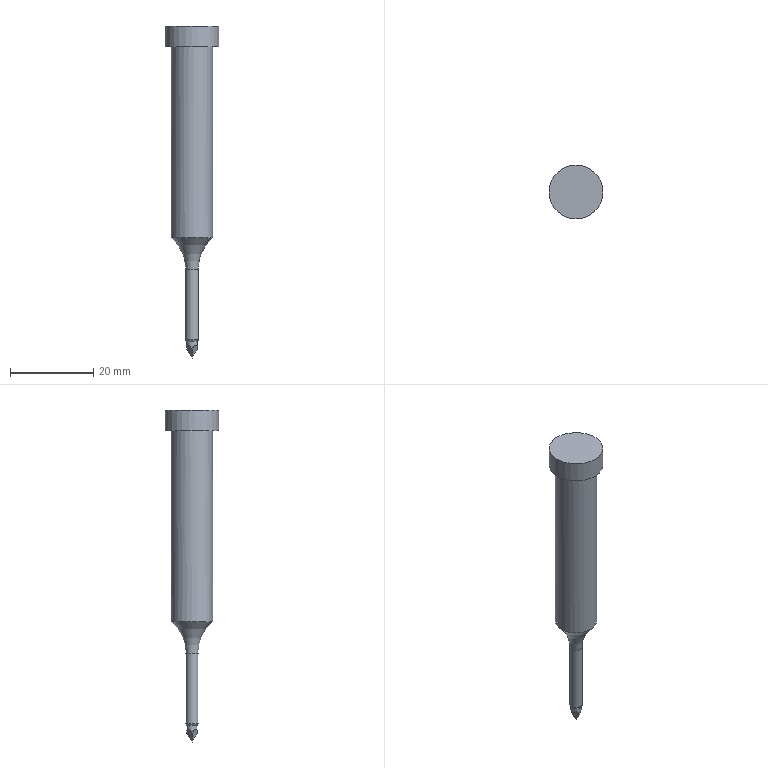Part | NX | features solid 2 | 1 solid | 13 faces | box 13 x 13 x 80 mm | volume 4592 mm3 | plane 7 | cylinder 4 | torus 2 | commonest cylinder face diameters 2.5 x1 3.006 x1 10 x1 13 x1
STEP:
#1=CARTESIAN_POINT('',(516.232,-362.056,-63.597));
#2=VERTEX_POINT('',#1);
#3=CARTESIAN_POINT('',(517.735,-362.056,-63.597));
#4=DIRECTION('',(0.,0.,-1.));
#5=DIRECTION('',(-1.,0.,0.));
#6=AXIS2_PLACEMENT_3D('',#3,#4,#5);
#7=CIRCLE('',#6,1.503);
#8=EDGE_CURVE('',#2,#2,#7,.F.);
#9=ORIENTED_EDGE('',*,*,#8,.F.);
#10=EDGE_LOOP('',(#9));
#11=FACE_BOUND('',#10,.T.);
#12=CARTESIAN_POINT('',(519.238,-362.056,-80.5));
#13=VERTEX_POINT('',#12);
#14=CARTESIAN_POINT('',(517.735,-362.056,-80.5));
#15=DIRECTION('',(0.,0.,1.));
#16=DIRECTION('',(1.,0.,0.));
#17=AXIS2_PLACEMENT_3D('',#14,#15,#16);
#18=CIRCLE('',#17,1.503);
#19=EDGE_CURVE('',#13,#13,#18,.F.);
#20=ORIENTED_EDGE('',*,*,#19,.F.);
#21=EDGE_LOOP('',(#20));
#22=FACE_BOUND('',#21,.T.);
#23=CARTESIAN_POINT('',(517.735,-362.056,-60.));
#24=DIRECTION('',(0.,0.,-1.));
#25=DIRECTION('',(1.,0.,0.));
#26=AXIS2_PLACEMENT_3D('',#23,#24,#25);
#27=CYLINDRICAL_SURFACE('',#26,1.503);
#28=ADVANCED_FACE('',(#11,#22),#27,.T.);
#29=ORIENTED_EDGE('',*,*,#19,.T.);
#30=EDGE_LOOP('',(#29));
#31=FACE_BOUND('',#30,.T.);
#32=CARTESIAN_POINT('',(518.738,-362.056,-81.));
#33=VERTEX_POINT('',#32);
#34=CARTESIAN_POINT('',(517.735,-362.056,-81.));
#35=DIRECTION('',(0.,0.,1.));
#36=DIRECTION('',(1.,0.,0.));
#37=AXIS2_PLACEMENT_3D('',#34,#35,#36);
#38=CIRCLE('',#37,1.003);
#39=EDGE_CURVE('',#33,#33,#38,.T.);
#40=ORIENTED_EDGE('',*,*,#39,.T.);
#41=EDGE_LOOP('',(#40));
#42=FACE_BOUND('',#41,.T.);
#43=CARTESIAN_POINT('',(517.735,-362.056,-80.5));
#44=DIRECTION('',(0.,0.,-1.));
#45=DIRECTION('',(1.,0.,0.));
#46=AXIS2_PLACEMENT_3D('',#43,#44,#45);
#47=TOROIDAL_SURFACE('',#46,1.003,0.5);
#48=ADVANCED_FACE('',(#31,#42),#47,.T.);
#49=CARTESIAN_POINT('',(522.735,-362.056,-56.));
#50=VERTEX_POINT('',#49);
#51=CARTESIAN_POINT('',(517.735,-362.056,-56.));
#52=DIRECTION('',(0.,0.,1.));
#53=DIRECTION('',(1.,0.,0.));
#54=AXIS2_PLACEMENT_3D('',#51,#52,#53);
#55=CIRCLE('',#54,5.);
#56=EDGE_CURVE('',#50,#50,#55,.T.);
#57=ORIENTED_EDGE('',*,*,#56,.F.);
#58=EDGE_LOOP('',(#57));
#59=FACE_BOUND('',#58,.T.);
#60=ORIENTED_EDGE('',*,*,#8,.T.);
#61=EDGE_LOOP('',(#60));
#62=FACE_BOUND('',#61,.T.);
#63=CARTESIAN_POINT('',(517.735,-362.056,-63.597));
#64=DIRECTION('',(0.,0.,1.));
#65=DIRECTION('',(-1.,0.,0.));
#66=AXIS2_PLACEMENT_3D('',#63,#64,#65);
#67=TOROIDAL_SURFACE('',#66,11.503,10.);
#68=ADVANCED_FACE('',(#59,#62),#67,.F.);
#69=CARTESIAN_POINT('',(518.985,-362.056,-81.));
#70=VERTEX_POINT('',#69);
#71=CARTESIAN_POINT('',(517.735,-362.056,-81.));
#72=DIRECTION('',(0.,0.,1.));
#73=DIRECTION('',(1.,0.,0.));
#74=AXIS2_PLACEMENT_3D('',#71,#72,#73);
#75=CIRCLE('',#74,1.25);
#76=EDGE_CURVE('',#70,#70,#75,.T.);
#77=ORIENTED_EDGE('',*,*,#76,.F.);
#78=EDGE_LOOP('',(#77));
#79=FACE_BOUND('',#78,.T.);
#80=CARTESIAN_POINT('',(518.985,-362.056,-82.835));
#81=VERTEX_POINT('',#80);
#82=CARTESIAN_POINT('',(517.735,-363.306,-82.835));
#83=VERTEX_POINT('',#82);
#84=CARTESIAN_POINT('',(517.735,-362.056,-85.));
#85=DIRECTION('',(0.6547,-0.6547,-0.378));
#86=DIRECTION('',(0.2673,-0.2673,0.9258));
#87=AXIS2_PLACEMENT_3D('',#84,#85,#86);
#88=ELLIPSE('',#87,3.307,1.25);
#89=EDGE_CURVE('',#81,#83,#88,.T.);
#90=ORIENTED_EDGE('',*,*,#89,.F.);
#91=CARTESIAN_POINT('',(517.735,-360.806,-82.835));
#92=VERTEX_POINT('',#91);
#93=CARTESIAN_POINT('',(517.735,-362.056,-85.));
#94=DIRECTION('',(0.6547,0.6547,-0.378));
#95=DIRECTION('',(0.2673,0.2673,0.9258));
#96=AXIS2_PLACEMENT_3D('',#93,#94,#95);
#97=ELLIPSE('',#96,3.307,1.25);
#98=EDGE_CURVE('',#92,#81,#97,.T.);
#99=ORIENTED_EDGE('',*,*,#98,.F.);
#100=CARTESIAN_POINT('',(516.485,-362.056,-82.835));
#101=VERTEX_POINT('',#100);
#102=CARTESIAN_POINT('',(517.735,-362.056,-85.));
#103=DIRECTION('',(0.6547,-0.6547,0.378));
#104=DIRECTION('',(-0.2673,0.2673,0.9258));
#105=AXIS2_PLACEMENT_3D('',#102,#103,#104);
#106=ELLIPSE('',#105,3.307,1.25);
#107=EDGE_CURVE('',#92,#101,#106,.T.);
#108=ORIENTED_EDGE('',*,*,#107,.T.);
#109=CARTESIAN_POINT('',(517.735,-362.056,-85.));
#110=DIRECTION('',(-0.6547,-0.6547,-0.378));
#111=DIRECTION('',(-0.2673,-0.2673,0.9258));
#112=AXIS2_PLACEMENT_3D('',#109,#110,#111);
#113=ELLIPSE('',#112,3.307,1.25);
#114=EDGE_CURVE('',#83,#101,#113,.T.);
#115=ORIENTED_EDGE('',*,*,#114,.F.);
#116=EDGE_LOOP('',(#90,#99,#108,#115));
#117=FACE_BOUND('',#116,.T.);
#118=CARTESIAN_POINT('',(517.735,-362.056,-85.));
#119=DIRECTION('',(0.,0.,1.));
#120=DIRECTION('',(-1.,0.,0.));
#121=AXIS2_PLACEMENT_3D('',#118,#119,#120);
#122=CYLINDRICAL_SURFACE('',#121,1.25);
#123=ADVANCED_FACE('',(#79,#117),#122,.T.);
#124=ORIENTED_EDGE('',*,*,#39,.F.);
#125=EDGE_LOOP('',(#124));
#126=FACE_BOUND('',#125,.T.);
#127=ORIENTED_EDGE('',*,*,#76,.T.);
#128=EDGE_LOOP('',(#127));
#129=FACE_BOUND('',#128,.T.);
#130=CARTESIAN_POINT('',(517.735,-362.056,-81.));
#131=DIRECTION('',(0.,0.,-1.));
#132=DIRECTION('',(1.,0.,0.));
#133=AXIS2_PLACEMENT_3D('',#130,#131,#132);
#134=PLANE('',#133);
#135=ADVANCED_FACE('',(#126,#129),#134,.F.);
#136=CARTESIAN_POINT('',(517.735,-362.056,-85.));
#137=VERTEX_POINT('',#136);
#138=CARTESIAN_POINT('',(517.735,-362.056,-85.));
#139=DIRECTION('',(0.5,0.,0.866));
#140=VECTOR('',#139,1000.);
#141=LINE('',#138,#140);
#142=EDGE_CURVE('',#81,#137,#141,.F.);
#143=ORIENTED_EDGE('',*,*,#142,.F.);
#144=ORIENTED_EDGE('',*,*,#89,.T.);
#145=CARTESIAN_POINT('',(517.735,-362.056,-85.));
#146=DIRECTION('',(0.,0.5,-0.866));
#147=VECTOR('',#146,1000.);
#148=LINE('',#145,#147);
#149=EDGE_CURVE('',#137,#83,#148,.F.);
#150=ORIENTED_EDGE('',*,*,#149,.F.);
#151=EDGE_LOOP('',(#143,#144,#150));
#152=FACE_BOUND('',#151,.T.);
#153=CARTESIAN_POINT('',(517.735,-362.056,-85.));
#154=DIRECTION('',(-0.6547,0.6547,0.378));
#155=DIRECTION('',(-0.7071,-0.7071,0.));
#156=AXIS2_PLACEMENT_3D('',#153,#154,#155);
#157=PLANE('',#156);
#158=ADVANCED_FACE('',(#152),#157,.F.);
#159=CARTESIAN_POINT('',(517.735,-362.056,-85.));
#160=DIRECTION('',(0.,0.5,0.866));
#161=VECTOR('',#160,1000.);
#162=LINE('',#159,#161);
#163=EDGE_CURVE('',#92,#137,#162,.F.);
#164=ORIENTED_EDGE('',*,*,#163,.F.);
#165=ORIENTED_EDGE('',*,*,#98,.T.);
#166=ORIENTED_EDGE('',*,*,#142,.T.);
#167=EDGE_LOOP('',(#164,#165,#166));
#168=FACE_BOUND('',#167,.T.);
#169=CARTESIAN_POINT('',(517.735,-362.056,-85.));
#170=DIRECTION('',(-0.6547,-0.6547,0.378));
#171=DIRECTION('',(0.7071,-0.7071,0.));
#172=AXIS2_PLACEMENT_3D('',#169,#170,#171);
#173=PLANE('',#172);
#174=ADVANCED_FACE('',(#168),#173,.F.);
#175=ORIENTED_EDGE('',*,*,#163,.T.);
#176=CARTESIAN_POINT('',(517.735,-362.056,-85.));
#177=DIRECTION('',(0.5,0.,-0.866));
#178=VECTOR('',#177,1000.);
#179=LINE('',#176,#178);
#180=EDGE_CURVE('',#137,#101,#179,.F.);
#181=ORIENTED_EDGE('',*,*,#180,.T.);
#182=ORIENTED_EDGE('',*,*,#107,.F.);
#183=EDGE_LOOP('',(#175,#181,#182));
#184=FACE_BOUND('',#183,.T.);
#185=CARTESIAN_POINT('',(517.735,-362.056,-85.));
#186=DIRECTION('',(-0.6547,0.6547,-0.378));
#187=DIRECTION('',(-0.7071,-0.7071,0.));
#188=AXIS2_PLACEMENT_3D('',#185,#186,#187);
#189=PLANE('',#188);
#190=ADVANCED_FACE('',(#184),#189,.T.);
#191=ORIENTED_EDGE('',*,*,#149,.T.);
#192=ORIENTED_EDGE('',*,*,#114,.T.);
#193=ORIENTED_EDGE('',*,*,#180,.F.);
#194=EDGE_LOOP('',(#191,#192,#193));
#195=FACE_BOUND('',#194,.T.);
#196=CARTESIAN_POINT('',(517.735,-362.056,-85.));
#197=DIRECTION('',(0.6547,0.6547,0.378));
#198=DIRECTION('',(-0.7071,0.7071,0.));
#199=AXIS2_PLACEMENT_3D('',#196,#197,#198);
#200=PLANE('',#199);
#201=ADVANCED_FACE('',(#195),#200,.F.);
#202=CARTESIAN_POINT('',(517.735,-357.056,-10.));
#203=VERTEX_POINT('',#202);
#204=CARTESIAN_POINT('',(517.735,-362.056,-10.));
#205=DIRECTION('',(0.,0.,1.));
#206=DIRECTION('',(0.,1.,0.));
#207=AXIS2_PLACEMENT_3D('',#204,#205,#206);
#208=CIRCLE('',#207,5.);
#209=EDGE_CURVE('',#203,#203,#208,.T.);
#210=ORIENTED_EDGE('',*,*,#209,.F.);
#211=EDGE_LOOP('',(#210));
#212=FACE_BOUND('',#211,.T.);
#213=ORIENTED_EDGE('',*,*,#56,.T.);
#214=EDGE_LOOP('',(#213));
#215=FACE_BOUND('',#214,.T.);
#216=CARTESIAN_POINT('',(517.735,-362.056,-5.));
#217=DIRECTION('',(0.,0.,-1.));
#218=DIRECTION('',(0.,-1.,0.));
#219=AXIS2_PLACEMENT_3D('',#216,#217,#218);
#220=CYLINDRICAL_SURFACE('',#219,5.);
#221=ADVANCED_FACE('',(#212,#215),#220,.T.);
#222=CARTESIAN_POINT('',(517.735,-355.556,-10.));
#223=VERTEX_POINT('',#222);
#224=CARTESIAN_POINT('',(517.735,-362.056,-10.));
#225=DIRECTION('',(0.,0.,1.));
#226=DIRECTION('',(0.,1.,0.));
#227=AXIS2_PLACEMENT_3D('',#224,#225,#226);
#228=CIRCLE('',#227,6.5);
#229=EDGE_CURVE('',#223,#223,#228,.T.);
#230=ORIENTED_EDGE('',*,*,#229,.F.);
#231=EDGE_LOOP('',(#230));
#232=FACE_BOUND('',#231,.T.);
#233=ORIENTED_EDGE('',*,*,#209,.T.);
#234=EDGE_LOOP('',(#233));
#235=FACE_BOUND('',#234,.T.);
#236=CARTESIAN_POINT('',(517.735,-362.056,-10.));
#237=DIRECTION('',(0.,0.,1.));
#238=DIRECTION('',(0.,1.,0.));
#239=AXIS2_PLACEMENT_3D('',#236,#237,#238);
#240=PLANE('',#239);
#241=ADVANCED_FACE('',(#232,#235),#240,.F.);
#242=ORIENTED_EDGE('',*,*,#229,.T.);
#243=EDGE_LOOP('',(#242));
#244=FACE_BOUND('',#243,.T.);
#245=CARTESIAN_POINT('',(517.735,-355.556,-5.));
#246=VERTEX_POINT('',#245);
#247=CARTESIAN_POINT('',(517.735,-362.056,-5.));
#248=DIRECTION('',(0.,0.,1.));
#249=DIRECTION('',(0.,1.,0.));
#250=AXIS2_PLACEMENT_3D('',#247,#248,#249);
#251=CIRCLE('',#250,6.5);
#252=EDGE_CURVE('',#246,#246,#251,.T.);
#253=ORIENTED_EDGE('',*,*,#252,.F.);
#254=EDGE_LOOP('',(#253));
#255=FACE_BOUND('',#254,.T.);
#256=CARTESIAN_POINT('',(517.735,-362.056,-10.));
#257=DIRECTION('',(0.,0.,1.));
#258=DIRECTION('',(0.,1.,0.));
#259=AXIS2_PLACEMENT_3D('',#256,#257,#258);
#260=CYLINDRICAL_SURFACE('',#259,6.5);
#261=ADVANCED_FACE('',(#244,#255),#260,.T.);
#262=ORIENTED_EDGE('',*,*,#252,.T.);
#263=EDGE_LOOP('',(#262));
#264=FACE_BOUND('',#263,.T.);
#265=CARTESIAN_POINT('',(517.735,-362.056,-5.));
#266=DIRECTION('',(0.,0.,1.));
#267=DIRECTION('',(0.,1.,0.));
#268=AXIS2_PLACEMENT_3D('',#265,#266,#267);
#269=PLANE('',#268);
#270=ADVANCED_FACE('',(#264),#269,.T.);
#271=CLOSED_SHELL('',(#28,#48,#68,#123,#135,#158,#174,#190,#201,#221,#241,#261,#270));
#272=MANIFOLD_SOLID_BREP('',#271);
#273=(LENGTH_UNIT()NAMED_UNIT(*)SI_UNIT(.MILLI.,.METRE.));
#274=UNCERTAINTY_MEASURE_WITH_UNIT(LENGTH_MEASURE(0.00001),#273,'','');
#275=(NAMED_UNIT(*)PLANE_ANGLE_UNIT()SI_UNIT($,.RADIAN.));
#276=(NAMED_UNIT(*)SI_UNIT($,.STERADIAN.)SOLID_ANGLE_UNIT());
#277=(GEOMETRIC_REPRESENTATION_CONTEXT(3)GLOBAL_UNCERTAINTY_ASSIGNED_CONTEXT((#274))GLOBAL_UNIT_ASSIGNED_CONTEXT((#273,#275,#276))REPRESENTATION_CONTEXT('',''));
#278=ADVANCED_BREP_SHAPE_REPRESENTATION('',(#272),#277);